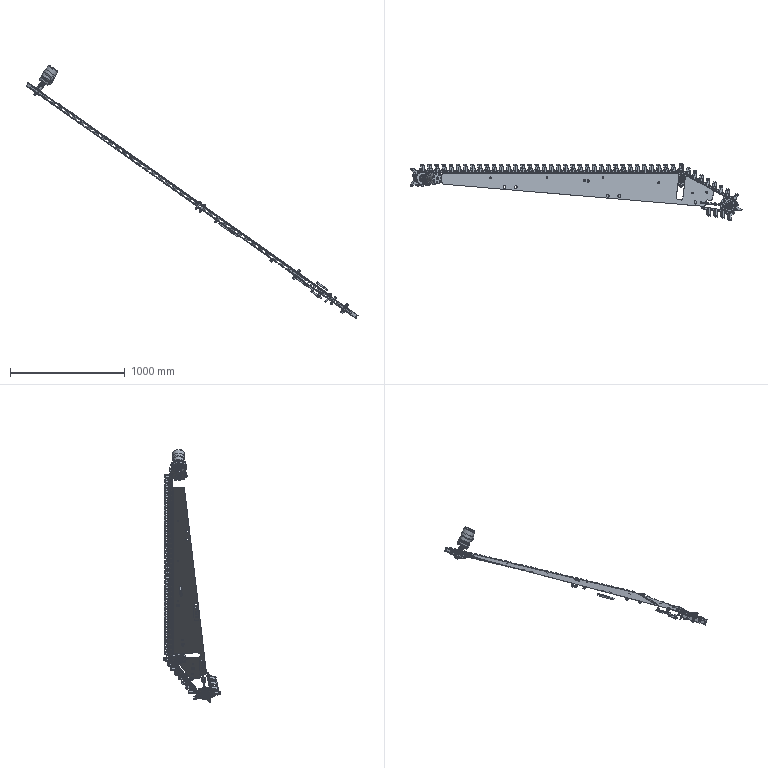Part | STEP file | COMPOUND | 183 solids | 4131 faces | volume 4143226 mm3 | plane 2036 | cylinder 1644 | cone 357 | torus 87 | spline 6 | sphere 1 | commonest cylinder face diameters 18 x424 6 x416 20 x175 12 x119 4 x105 16 x82